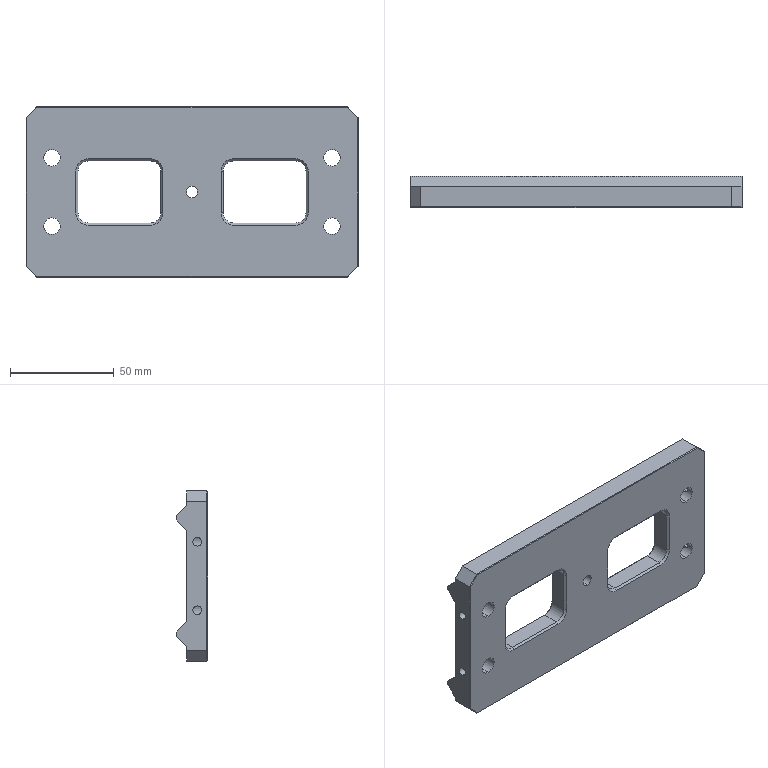Part | STEP file | lifting air cylinder fixing support seat 02 | 1 solid | 95 faces | box 160 x 15 x 82 mm | volume 115095 mm3 | plane 51 | cylinder 28 | cone 16 | commonest cylinder face diameters 4.2 x8 8 x8 10 x8 5.5 x2 9 x2